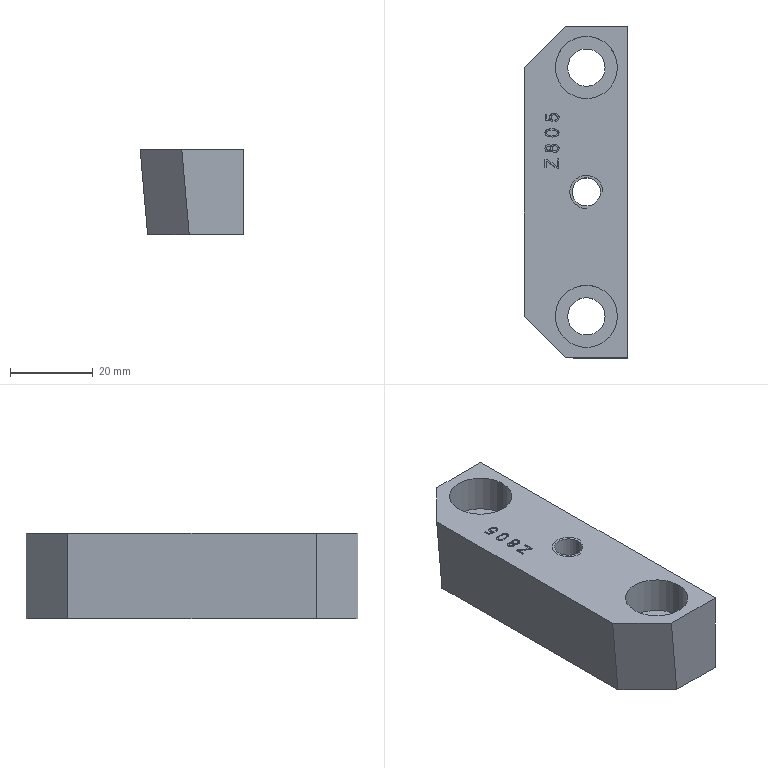Part | Creo | 2 solids | 116 faces | box 25 x 80 x 20.5 mm | volume 32081 mm3 | other 73 | plane 29 | cylinder 14 | commonest cylinder face diameters 9 x4 15 x4 6.8 x2 1.666 x1 7.998 x1 8 x1